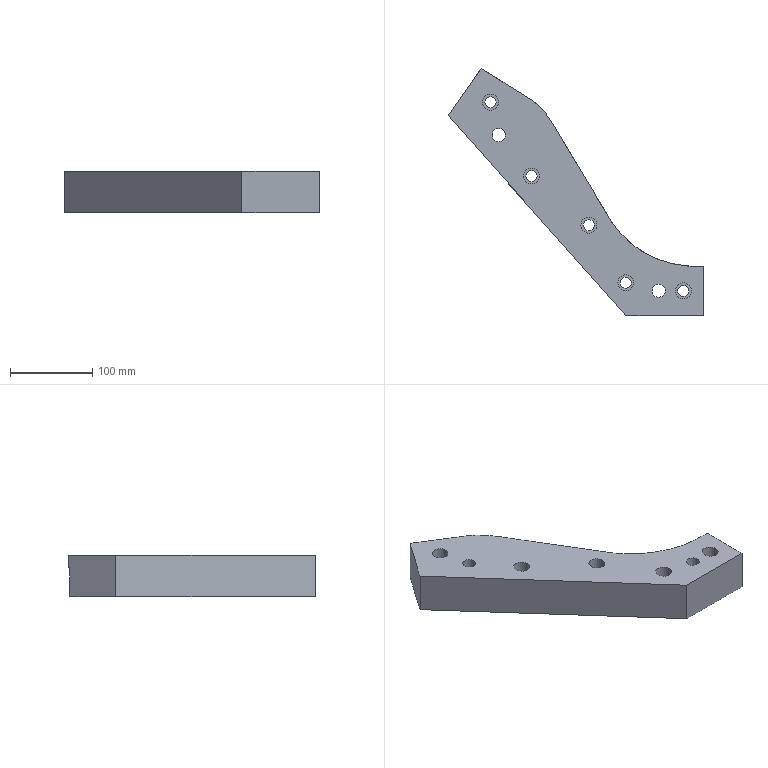Part | NX | features solid 2 | 1 solid | 26 faces | box 311.506 x 301.101 x 50 mm | volume 1333473 mm3 | cylinder 12 | plane 11 | spline 3 | commonest cylinder face diameters 13.5 x5 19.5 x5 16 x2